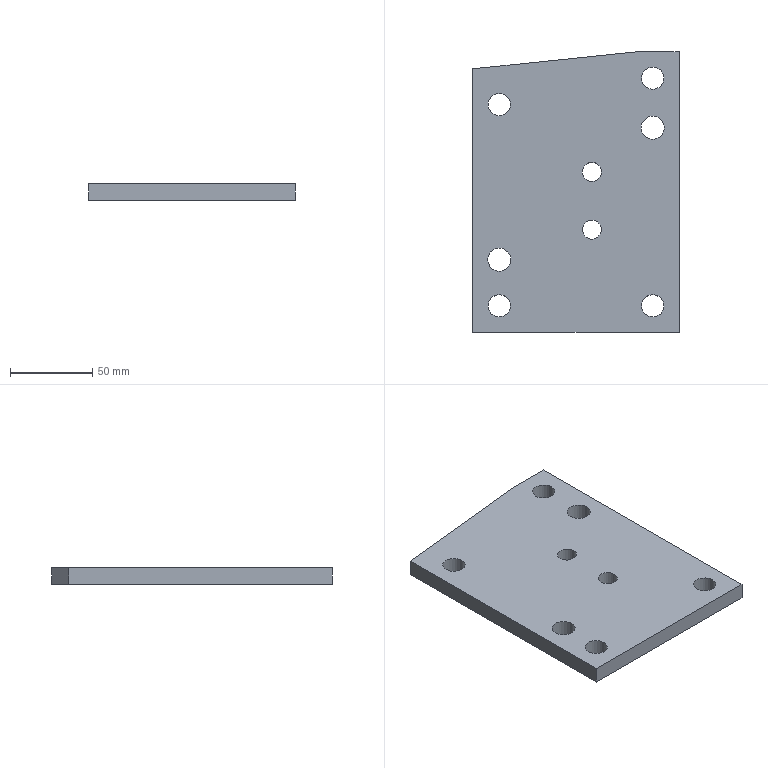Part | STEP file | lll_id2954_x_t | 1 solid | 15 faces | box 125 x 170 x 10 mm | volume 196494 mm3 | cylinder 8 | plane 7 | commonest cylinder face diameters 13.509 x4 11.5 x2 14 x2
STEP:
#1=CARTESIAN_POINT('',(403.893,-140.43,102.5));
#2=VERTEX_POINT('',#1);
#3=CARTESIAN_POINT('',(410.893,-140.43,102.5));
#4=DIRECTION('',(0.,0.,1.));
#5=DIRECTION('',(-1.,0.,0.));
#6=AXIS2_PLACEMENT_3D('',#3,#4,#5);
#7=CIRCLE('',#6,7.);
#8=EDGE_CURVE('',#2,#2,#7,.T.);
#9=ORIENTED_EDGE('',*,*,#8,.T.);
#10=EDGE_LOOP('',(#9));
#11=FACE_BOUND('',#10,.T.);
#12=CARTESIAN_POINT('',(403.893,-140.43,92.5));
#13=VERTEX_POINT('',#12);
#14=CARTESIAN_POINT('',(410.893,-140.43,92.5));
#15=DIRECTION('',(0.,0.,1.));
#16=DIRECTION('',(-1.,0.,0.));
#17=AXIS2_PLACEMENT_3D('',#14,#15,#16);
#18=CIRCLE('',#17,7.);
#19=EDGE_CURVE('',#13,#13,#18,.T.);
#20=ORIENTED_EDGE('',*,*,#19,.F.);
#21=EDGE_LOOP('',(#20));
#22=FACE_BOUND('',#21,.T.);
#23=CARTESIAN_POINT('',(410.893,-140.43,92.5));
#24=DIRECTION('',(0.,0.,1.));
#25=DIRECTION('',(-1.,0.,0.));
#26=AXIS2_PLACEMENT_3D('',#23,#24,#25);
#27=CYLINDRICAL_SURFACE('',#26,7.);
#28=ADVANCED_FACE('',(#11,#22),#27,.F.);
#29=CARTESIAN_POINT('',(497.138,-168.43,102.5));
#30=VERTEX_POINT('',#29);
#31=CARTESIAN_POINT('',(503.893,-168.43,102.5));
#32=DIRECTION('',(0.,0.,1.));
#33=DIRECTION('',(-1.,0.,0.));
#34=AXIS2_PLACEMENT_3D('',#31,#32,#33);
#35=CIRCLE('',#34,6.755);
#36=EDGE_CURVE('',#30,#30,#35,.T.);
#37=ORIENTED_EDGE('',*,*,#36,.T.);
#38=EDGE_LOOP('',(#37));
#39=FACE_BOUND('',#38,.T.);
#40=CARTESIAN_POINT('',(497.138,-168.43,92.5));
#41=VERTEX_POINT('',#40);
#42=CARTESIAN_POINT('',(503.893,-168.43,92.5));
#43=DIRECTION('',(0.,0.,1.));
#44=DIRECTION('',(-1.,0.,0.));
#45=AXIS2_PLACEMENT_3D('',#42,#43,#44);
#46=CIRCLE('',#45,6.755);
#47=EDGE_CURVE('',#41,#41,#46,.T.);
#48=ORIENTED_EDGE('',*,*,#47,.F.);
#49=EDGE_LOOP('',(#48));
#50=FACE_BOUND('',#49,.T.);
#51=CARTESIAN_POINT('',(503.893,-168.43,92.5));
#52=DIRECTION('',(0.,0.,1.));
#53=DIRECTION('',(-1.,0.,0.));
#54=AXIS2_PLACEMENT_3D('',#51,#52,#53);
#55=CYLINDRICAL_SURFACE('',#54,6.755);
#56=ADVANCED_FACE('',(#39,#50),#55,.F.);
#57=CARTESIAN_POINT('',(404.138,-168.43,102.5));
#58=VERTEX_POINT('',#57);
#59=CARTESIAN_POINT('',(410.893,-168.43,102.5));
#60=DIRECTION('',(0.,0.,-1.));
#61=DIRECTION('',(-1.,0.,0.));
#62=AXIS2_PLACEMENT_3D('',#59,#60,#61);
#63=CIRCLE('',#62,6.755);
#64=EDGE_CURVE('',#58,#58,#63,.T.);
#65=ORIENTED_EDGE('',*,*,#64,.F.);
#66=EDGE_LOOP('',(#65));
#67=FACE_BOUND('',#66,.T.);
#68=CARTESIAN_POINT('',(404.138,-168.43,92.5));
#69=VERTEX_POINT('',#68);
#70=CARTESIAN_POINT('',(410.893,-168.43,92.5));
#71=DIRECTION('',(0.,0.,1.));
#72=DIRECTION('',(-1.,0.,0.));
#73=AXIS2_PLACEMENT_3D('',#70,#71,#72);
#74=CIRCLE('',#73,6.755);
#75=EDGE_CURVE('',#69,#69,#74,.T.);
#76=ORIENTED_EDGE('',*,*,#75,.F.);
#77=EDGE_LOOP('',(#76));
#78=FACE_BOUND('',#77,.T.);
#79=CARTESIAN_POINT('',(410.893,-168.43,92.5));
#80=DIRECTION('',(0.,0.,1.));
#81=DIRECTION('',(-1.,0.,0.));
#82=AXIS2_PLACEMENT_3D('',#79,#80,#81);
#83=CYLINDRICAL_SURFACE('',#82,6.755);
#84=ADVANCED_FACE('',(#67,#78),#83,.F.);
#85=CARTESIAN_POINT('',(497.138,-30.43,102.5));
#86=VERTEX_POINT('',#85);
#87=CARTESIAN_POINT('',(503.893,-30.43,102.5));
#88=DIRECTION('',(0.,0.,-1.));
#89=DIRECTION('',(-1.,0.,0.));
#90=AXIS2_PLACEMENT_3D('',#87,#88,#89);
#91=CIRCLE('',#90,6.755);
#92=EDGE_CURVE('',#86,#86,#91,.T.);
#93=ORIENTED_EDGE('',*,*,#92,.F.);
#94=EDGE_LOOP('',(#93));
#95=FACE_BOUND('',#94,.T.);
#96=CARTESIAN_POINT('',(497.138,-30.43,92.5));
#97=VERTEX_POINT('',#96);
#98=CARTESIAN_POINT('',(503.893,-30.43,92.5));
#99=DIRECTION('',(0.,0.,1.));
#100=DIRECTION('',(-1.,0.,0.));
#101=AXIS2_PLACEMENT_3D('',#98,#99,#100);
#102=CIRCLE('',#101,6.755);
#103=EDGE_CURVE('',#97,#97,#102,.T.);
#104=ORIENTED_EDGE('',*,*,#103,.F.);
#105=EDGE_LOOP('',(#104));
#106=FACE_BOUND('',#105,.T.);
#107=CARTESIAN_POINT('',(503.893,-30.43,92.5));
#108=DIRECTION('',(0.,0.,1.));
#109=DIRECTION('',(-1.,0.,0.));
#110=AXIS2_PLACEMENT_3D('',#107,#108,#109);
#111=CYLINDRICAL_SURFACE('',#110,6.755);
#112=ADVANCED_FACE('',(#95,#106),#111,.F.);
#113=CARTESIAN_POINT('',(404.138,-46.43,102.5));
#114=VERTEX_POINT('',#113);
#115=CARTESIAN_POINT('',(410.893,-46.43,102.5));
#116=DIRECTION('',(0.,0.,1.));
#117=DIRECTION('',(-1.,0.,0.));
#118=AXIS2_PLACEMENT_3D('',#115,#116,#117);
#119=CIRCLE('',#118,6.755);
#120=EDGE_CURVE('',#114,#114,#119,.T.);
#121=ORIENTED_EDGE('',*,*,#120,.T.);
#122=EDGE_LOOP('',(#121));
#123=FACE_BOUND('',#122,.T.);
#124=CARTESIAN_POINT('',(404.138,-46.43,92.5));
#125=VERTEX_POINT('',#124);
#126=CARTESIAN_POINT('',(410.893,-46.43,92.5));
#127=DIRECTION('',(0.,0.,1.));
#128=DIRECTION('',(-1.,0.,0.));
#129=AXIS2_PLACEMENT_3D('',#126,#127,#128);
#130=CIRCLE('',#129,6.755);
#131=EDGE_CURVE('',#125,#125,#130,.T.);
#132=ORIENTED_EDGE('',*,*,#131,.F.);
#133=EDGE_LOOP('',(#132));
#134=FACE_BOUND('',#133,.T.);
#135=CARTESIAN_POINT('',(410.893,-46.43,92.5));
#136=DIRECTION('',(0.,0.,1.));
#137=DIRECTION('',(-1.,0.,0.));
#138=AXIS2_PLACEMENT_3D('',#135,#136,#137);
#139=CYLINDRICAL_SURFACE('',#138,6.755);
#140=ADVANCED_FACE('',(#123,#134),#139,.F.);
#141=CARTESIAN_POINT('',(496.893,-60.43,102.5));
#142=VERTEX_POINT('',#141);
#143=CARTESIAN_POINT('',(503.893,-60.43,102.5));
#144=DIRECTION('',(0.,0.,-1.));
#145=DIRECTION('',(-1.,0.,0.));
#146=AXIS2_PLACEMENT_3D('',#143,#144,#145);
#147=CIRCLE('',#146,7.);
#148=EDGE_CURVE('',#142,#142,#147,.T.);
#149=ORIENTED_EDGE('',*,*,#148,.F.);
#150=EDGE_LOOP('',(#149));
#151=FACE_BOUND('',#150,.T.);
#152=CARTESIAN_POINT('',(496.893,-60.43,92.5));
#153=VERTEX_POINT('',#152);
#154=CARTESIAN_POINT('',(503.893,-60.43,92.5));
#155=DIRECTION('',(0.,0.,1.));
#156=DIRECTION('',(-1.,0.,0.));
#157=AXIS2_PLACEMENT_3D('',#154,#155,#156);
#158=CIRCLE('',#157,7.);
#159=EDGE_CURVE('',#153,#153,#158,.T.);
#160=ORIENTED_EDGE('',*,*,#159,.F.);
#161=EDGE_LOOP('',(#160));
#162=FACE_BOUND('',#161,.T.);
#163=CARTESIAN_POINT('',(503.893,-60.43,92.5));
#164=DIRECTION('',(0.,0.,1.));
#165=DIRECTION('',(-1.,0.,0.));
#166=AXIS2_PLACEMENT_3D('',#163,#164,#165);
#167=CYLINDRICAL_SURFACE('',#166,7.);
#168=ADVANCED_FACE('',(#151,#162),#167,.F.);
#169=CARTESIAN_POINT('',(519.893,-184.43,102.5));
#170=VERTEX_POINT('',#169);
#171=CARTESIAN_POINT('',(394.893,-184.43,102.5));
#172=VERTEX_POINT('',#171);
#173=CARTESIAN_POINT('',(457.393,-184.43,102.5));
#174=DIRECTION('',(-1.,0.,0.));
#175=VECTOR('',#174,1.);
#176=LINE('',#173,#175);
#177=EDGE_CURVE('',#170,#172,#176,.T.);
#178=ORIENTED_EDGE('',*,*,#177,.T.);
#179=CARTESIAN_POINT('',(394.893,-184.43,92.5));
#180=VERTEX_POINT('',#179);
#181=CARTESIAN_POINT('',(394.893,-184.43,92.5));
#182=DIRECTION('',(0.,0.,1.));
#183=VECTOR('',#182,1.);
#184=LINE('',#181,#183);
#185=EDGE_CURVE('',#180,#172,#184,.T.);
#186=ORIENTED_EDGE('',*,*,#185,.F.);
#187=CARTESIAN_POINT('',(519.893,-184.43,92.5));
#188=VERTEX_POINT('',#187);
#189=CARTESIAN_POINT('',(457.393,-184.43,92.5));
#190=DIRECTION('',(1.,0.,0.));
#191=VECTOR('',#190,1.);
#192=LINE('',#189,#191);
#193=EDGE_CURVE('',#180,#188,#192,.T.);
#194=ORIENTED_EDGE('',*,*,#193,.T.);
#195=CARTESIAN_POINT('',(519.893,-184.43,92.5));
#196=DIRECTION('',(0.,0.,1.));
#197=VECTOR('',#196,1.);
#198=LINE('',#195,#197);
#199=EDGE_CURVE('',#188,#170,#198,.T.);
#200=ORIENTED_EDGE('',*,*,#199,.T.);
#201=EDGE_LOOP('',(#178,#186,#194,#200));
#202=FACE_OUTER_BOUND('',#201,.T.);
#203=CARTESIAN_POINT('',(457.393,-184.43,92.5));
#204=DIRECTION('',(0.,-1.,0.));
#205=DIRECTION('',(0.,0.,1.));
#206=AXIS2_PLACEMENT_3D('',#203,#204,#205);
#207=PLANE('',#206);
#208=ADVANCED_FACE('',(#202),#207,.T.);
#209=CARTESIAN_POINT('',(519.893,-14.43,102.5));
#210=VERTEX_POINT('',#209);
#211=CARTESIAN_POINT('',(519.893,-99.43,102.5));
#212=DIRECTION('',(0.,-1.,0.));
#213=VECTOR('',#212,1.);
#214=LINE('',#211,#213);
#215=EDGE_CURVE('',#210,#170,#214,.T.);
#216=ORIENTED_EDGE('',*,*,#215,.T.);
#217=ORIENTED_EDGE('',*,*,#199,.F.);
#218=CARTESIAN_POINT('',(519.893,-14.43,92.5));
#219=VERTEX_POINT('',#218);
#220=CARTESIAN_POINT('',(519.893,-99.43,92.5));
#221=DIRECTION('',(0.,1.,0.));
#222=VECTOR('',#221,1.);
#223=LINE('',#220,#222);
#224=EDGE_CURVE('',#188,#219,#223,.T.);
#225=ORIENTED_EDGE('',*,*,#224,.T.);
#226=CARTESIAN_POINT('',(519.893,-14.43,92.5));
#227=DIRECTION('',(0.,0.,1.));
#228=VECTOR('',#227,1.);
#229=LINE('',#226,#228);
#230=EDGE_CURVE('',#219,#210,#229,.T.);
#231=ORIENTED_EDGE('',*,*,#230,.T.);
#232=EDGE_LOOP('',(#216,#217,#225,#231));
#233=FACE_OUTER_BOUND('',#232,.T.);
#234=CARTESIAN_POINT('',(519.893,-99.43,92.5));
#235=DIRECTION('',(1.,0.,0.));
#236=DIRECTION('',(0.,0.,1.));
#237=AXIS2_PLACEMENT_3D('',#234,#235,#236);
#238=PLANE('',#237);
#239=ADVANCED_FACE('',(#233),#238,.T.);
#240=CARTESIAN_POINT('',(493.966,-14.43,102.5));
#241=VERTEX_POINT('',#240);
#242=CARTESIAN_POINT('',(394.893,-24.758,102.5));
#243=VERTEX_POINT('',#242);
#244=CARTESIAN_POINT('',(479.656,-15.922,102.5));
#245=DIRECTION('',(-0.9946,-0.1037,0.));
#246=VECTOR('',#245,1.);
#247=LINE('',#244,#246);
#248=EDGE_CURVE('',#241,#243,#247,.T.);
#249=ORIENTED_EDGE('',*,*,#248,.F.);
#250=CARTESIAN_POINT('',(493.966,-14.43,92.5));
#251=VERTEX_POINT('',#250);
#252=CARTESIAN_POINT('',(493.966,-14.43,-1360.5));
#253=DIRECTION('',(0.,0.,-1.));
#254=VECTOR('',#253,1.);
#255=LINE('',#252,#254);
#256=EDGE_CURVE('',#241,#251,#255,.T.);
#257=ORIENTED_EDGE('',*,*,#256,.T.);
#258=CARTESIAN_POINT('',(394.893,-24.758,92.5));
#259=VERTEX_POINT('',#258);
#260=CARTESIAN_POINT('',(479.656,-15.922,92.5));
#261=DIRECTION('',(-0.9946,-0.1037,0.));
#262=VECTOR('',#261,1.);
#263=LINE('',#260,#262);
#264=EDGE_CURVE('',#251,#259,#263,.T.);
#265=ORIENTED_EDGE('',*,*,#264,.T.);
#266=CARTESIAN_POINT('',(394.893,-24.758,-1360.5));
#267=DIRECTION('',(0.,0.,1.));
#268=VECTOR('',#267,1.);
#269=LINE('',#266,#268);
#270=EDGE_CURVE('',#259,#243,#269,.T.);
#271=ORIENTED_EDGE('',*,*,#270,.T.);
#272=EDGE_LOOP('',(#249,#257,#265,#271));
#273=FACE_OUTER_BOUND('',#272,.T.);
#274=CARTESIAN_POINT('',(479.656,-15.922,-1360.5));
#275=DIRECTION('',(-0.1037,0.9946,0.));
#276=DIRECTION('',(-0.9946,-0.1037,0.));
#277=AXIS2_PLACEMENT_3D('',#274,#275,#276);
#278=PLANE('',#277);
#279=ADVANCED_FACE('',(#273),#278,.T.);
#280=CARTESIAN_POINT('',(394.893,-99.43,102.5));
#281=DIRECTION('',(0.,-1.,0.));
#282=VECTOR('',#281,1.);
#283=LINE('',#280,#282);
#284=EDGE_CURVE('',#243,#172,#283,.T.);
#285=ORIENTED_EDGE('',*,*,#284,.F.);
#286=ORIENTED_EDGE('',*,*,#270,.F.);
#287=CARTESIAN_POINT('',(394.893,-99.43,92.5));
#288=DIRECTION('',(0.,-1.,0.));
#289=VECTOR('',#288,1.);
#290=LINE('',#287,#289);
#291=EDGE_CURVE('',#259,#180,#290,.T.);
#292=ORIENTED_EDGE('',*,*,#291,.T.);
#293=ORIENTED_EDGE('',*,*,#185,.T.);
#294=EDGE_LOOP('',(#285,#286,#292,#293));
#295=FACE_OUTER_BOUND('',#294,.T.);
#296=CARTESIAN_POINT('',(394.893,-99.43,92.5));
#297=DIRECTION('',(-1.,0.,0.));
#298=DIRECTION('',(0.,0.,-1.));
#299=AXIS2_PLACEMENT_3D('',#296,#297,#298);
#300=PLANE('',#299);
#301=ADVANCED_FACE('',(#295),#300,.T.);
#302=CARTESIAN_POINT('',(457.393,-14.43,102.5));
#303=DIRECTION('',(-1.,0.,0.));
#304=VECTOR('',#303,1.);
#305=LINE('',#302,#304);
#306=EDGE_CURVE('',#210,#241,#305,.T.);
#307=ORIENTED_EDGE('',*,*,#306,.F.);
#308=ORIENTED_EDGE('',*,*,#230,.F.);
#309=CARTESIAN_POINT('',(457.393,-14.43,92.5));
#310=DIRECTION('',(-1.,0.,0.));
#311=VECTOR('',#310,1.);
#312=LINE('',#309,#311);
#313=EDGE_CURVE('',#219,#251,#312,.T.);
#314=ORIENTED_EDGE('',*,*,#313,.T.);
#315=ORIENTED_EDGE('',*,*,#256,.F.);
#316=EDGE_LOOP('',(#307,#308,#314,#315));
#317=FACE_OUTER_BOUND('',#316,.T.);
#318=CARTESIAN_POINT('',(457.393,-14.43,92.5));
#319=DIRECTION('',(0.,1.,0.));
#320=DIRECTION('',(0.,0.,-1.));
#321=AXIS2_PLACEMENT_3D('',#318,#319,#320);
#322=PLANE('',#321);
#323=ADVANCED_FACE('',(#317),#322,.T.);
#324=CARTESIAN_POINT('',(461.25,-87.231,92.5));
#325=VERTEX_POINT('',#324);
#326=CARTESIAN_POINT('',(467.,-87.231,92.5));
#327=DIRECTION('',(0.,0.,-1.));
#328=DIRECTION('',(-1.,0.,0.));
#329=AXIS2_PLACEMENT_3D('',#326,#327,#328);
#330=CIRCLE('',#329,5.75);
#331=EDGE_CURVE('',#325,#325,#330,.T.);
#332=ORIENTED_EDGE('',*,*,#331,.F.);
#333=EDGE_LOOP('',(#332));
#334=FACE_BOUND('',#333,.T.);
#335=ORIENTED_EDGE('',*,*,#291,.F.);
#336=ORIENTED_EDGE('',*,*,#264,.F.);
#337=ORIENTED_EDGE('',*,*,#313,.F.);
#338=ORIENTED_EDGE('',*,*,#224,.F.);
#339=ORIENTED_EDGE('',*,*,#193,.F.);
#340=EDGE_LOOP('',(#335,#336,#337,#338,#339));
#341=FACE_BOUND('',#340,.T.);
#342=ORIENTED_EDGE('',*,*,#159,.T.);
#343=EDGE_LOOP('',(#342));
#344=FACE_BOUND('',#343,.T.);
#345=ORIENTED_EDGE('',*,*,#131,.T.);
#346=EDGE_LOOP('',(#345));
#347=FACE_BOUND('',#346,.T.);
#348=ORIENTED_EDGE('',*,*,#103,.T.);
#349=EDGE_LOOP('',(#348));
#350=FACE_BOUND('',#349,.T.);
#351=ORIENTED_EDGE('',*,*,#75,.T.);
#352=EDGE_LOOP('',(#351));
#353=FACE_BOUND('',#352,.T.);
#354=ORIENTED_EDGE('',*,*,#47,.T.);
#355=EDGE_LOOP('',(#354));
#356=FACE_BOUND('',#355,.T.);
#357=ORIENTED_EDGE('',*,*,#19,.T.);
#358=EDGE_LOOP('',(#357));
#359=FACE_BOUND('',#358,.T.);
#360=CARTESIAN_POINT('',(461.25,-122.231,92.5));
#361=VERTEX_POINT('',#360);
#362=CARTESIAN_POINT('',(467.,-122.231,92.5));
#363=DIRECTION('',(0.,0.,-1.));
#364=DIRECTION('',(-1.,0.,0.));
#365=AXIS2_PLACEMENT_3D('',#362,#363,#364);
#366=CIRCLE('',#365,5.75);
#367=EDGE_CURVE('',#361,#361,#366,.T.);
#368=ORIENTED_EDGE('',*,*,#367,.F.);
#369=EDGE_LOOP('',(#368));
#370=FACE_BOUND('',#369,.T.);
#371=CARTESIAN_POINT('',(457.393,-99.43,92.5));
#372=DIRECTION('',(0.,0.,-1.));
#373=DIRECTION('',(1.,0.,0.));
#374=AXIS2_PLACEMENT_3D('',#371,#372,#373);
#375=PLANE('',#374);
#376=ADVANCED_FACE('',(#334,#341,#344,#347,#350,#353,#356,#359,#370),#375,.T.);
#377=CARTESIAN_POINT('',(461.25,-87.231,102.5));
#378=VERTEX_POINT('',#377);
#379=CARTESIAN_POINT('',(467.,-87.231,102.5));
#380=DIRECTION('',(0.,0.,-1.));
#381=DIRECTION('',(-1.,0.,0.));
#382=AXIS2_PLACEMENT_3D('',#379,#380,#381);
#383=CIRCLE('',#382,5.75);
#384=EDGE_CURVE('',#378,#378,#383,.T.);
#385=ORIENTED_EDGE('',*,*,#384,.T.);
#386=EDGE_LOOP('',(#385));
#387=FACE_BOUND('',#386,.T.);
#388=CARTESIAN_POINT('',(461.25,-122.231,102.5));
#389=VERTEX_POINT('',#388);
#390=CARTESIAN_POINT('',(467.,-122.231,102.5));
#391=DIRECTION('',(0.,0.,-1.));
#392=DIRECTION('',(-1.,0.,0.));
#393=AXIS2_PLACEMENT_3D('',#390,#391,#392);
#394=CIRCLE('',#393,5.75);
#395=EDGE_CURVE('',#389,#389,#394,.T.);
#396=ORIENTED_EDGE('',*,*,#395,.T.);
#397=EDGE_LOOP('',(#396));
#398=FACE_BOUND('',#397,.T.);
#399=ORIENTED_EDGE('',*,*,#64,.T.);
#400=EDGE_LOOP('',(#399));
#401=FACE_BOUND('',#400,.T.);
#402=ORIENTED_EDGE('',*,*,#36,.F.);
#403=EDGE_LOOP('',(#402));
#404=FACE_BOUND('',#403,.T.);
#405=ORIENTED_EDGE('',*,*,#8,.F.);
#406=EDGE_LOOP('',(#405));
#407=FACE_BOUND('',#406,.T.);
#408=ORIENTED_EDGE('',*,*,#215,.F.);
#409=ORIENTED_EDGE('',*,*,#306,.T.);
#410=ORIENTED_EDGE('',*,*,#248,.T.);
#411=ORIENTED_EDGE('',*,*,#284,.T.);
#412=ORIENTED_EDGE('',*,*,#177,.F.);
#413=EDGE_LOOP('',(#408,#409,#410,#411,#412));
#414=FACE_BOUND('',#413,.T.);
#415=ORIENTED_EDGE('',*,*,#148,.T.);
#416=EDGE_LOOP('',(#415));
#417=FACE_BOUND('',#416,.T.);
#418=ORIENTED_EDGE('',*,*,#120,.F.);
#419=EDGE_LOOP('',(#418));
#420=FACE_BOUND('',#419,.T.);
#421=ORIENTED_EDGE('',*,*,#92,.T.);
#422=EDGE_LOOP('',(#421));
#423=FACE_BOUND('',#422,.T.);
#424=CARTESIAN_POINT('',(741.5,-0.002299,102.5));
#425=DIRECTION('',(0.,0.,-1.));
#426=DIRECTION('',(-1.,0.,0.));
#427=AXIS2_PLACEMENT_3D('',#424,#425,#426);
#428=PLANE('',#427);
#429=ADVANCED_FACE('',(#387,#398,#401,#404,#407,#414,#417,#420,#423),#428,.F.);
#430=ORIENTED_EDGE('',*,*,#367,.T.);
#431=EDGE_LOOP('',(#430));
#432=FACE_BOUND('',#431,.T.);
#433=ORIENTED_EDGE('',*,*,#395,.F.);
#434=EDGE_LOOP('',(#433));
#435=FACE_BOUND('',#434,.T.);
#436=CARTESIAN_POINT('',(467.,-122.231,-7.5));
#437=DIRECTION('',(0.,0.,1.));
#438=DIRECTION('',(1.,0.,0.));
#439=AXIS2_PLACEMENT_3D('',#436,#437,#438);
#440=CYLINDRICAL_SURFACE('',#439,5.75);
#441=ADVANCED_FACE('',(#432,#435),#440,.F.);
#442=ORIENTED_EDGE('',*,*,#331,.T.);
#443=EDGE_LOOP('',(#442));
#444=FACE_BOUND('',#443,.T.);
#445=ORIENTED_EDGE('',*,*,#384,.F.);
#446=EDGE_LOOP('',(#445));
#447=FACE_BOUND('',#446,.T.);
#448=CARTESIAN_POINT('',(467.,-87.231,-7.5));
#449=DIRECTION('',(0.,0.,1.));
#450=DIRECTION('',(1.,0.,0.));
#451=AXIS2_PLACEMENT_3D('',#448,#449,#450);
#452=CYLINDRICAL_SURFACE('',#451,5.75);
#453=ADVANCED_FACE('',(#444,#447),#452,.F.);
#454=CLOSED_SHELL('',(#28,#56,#84,#112,#140,#168,#208,#239,#279,#301,#323,#376,#429,#441,#453));
#455=MANIFOLD_SOLID_BREP('',#454);
#456=(LENGTH_UNIT()NAMED_UNIT(*)SI_UNIT(.MILLI.,.METRE.));
#457=UNCERTAINTY_MEASURE_WITH_UNIT(LENGTH_MEASURE(0.00002),#456,'','');
#458=(NAMED_UNIT(*)PLANE_ANGLE_UNIT()SI_UNIT($,.RADIAN.));
#459=PLANE_ANGLE_MEASURE_WITH_UNIT(PLANE_ANGLE_MEASURE(0.01745),#458);
#460=DIMENSIONAL_EXPONENTS(0.,0.,0.,0.,0.,0.,0.);
#461=(CONVERSION_BASED_UNIT('DEGREE',#459)NAMED_UNIT(#460)PLANE_ANGLE_UNIT());
#462=(NAMED_UNIT(*)SI_UNIT($,.STERADIAN.)SOLID_ANGLE_UNIT());
#463=(GEOMETRIC_REPRESENTATION_CONTEXT(3)GLOBAL_UNCERTAINTY_ASSIGNED_CONTEXT((#457))GLOBAL_UNIT_ASSIGNED_CONTEXT((#456,#461,#462))REPRESENTATION_CONTEXT('',''));
#464=ADVANCED_BREP_SHAPE_REPRESENTATION('',(#455),#463);